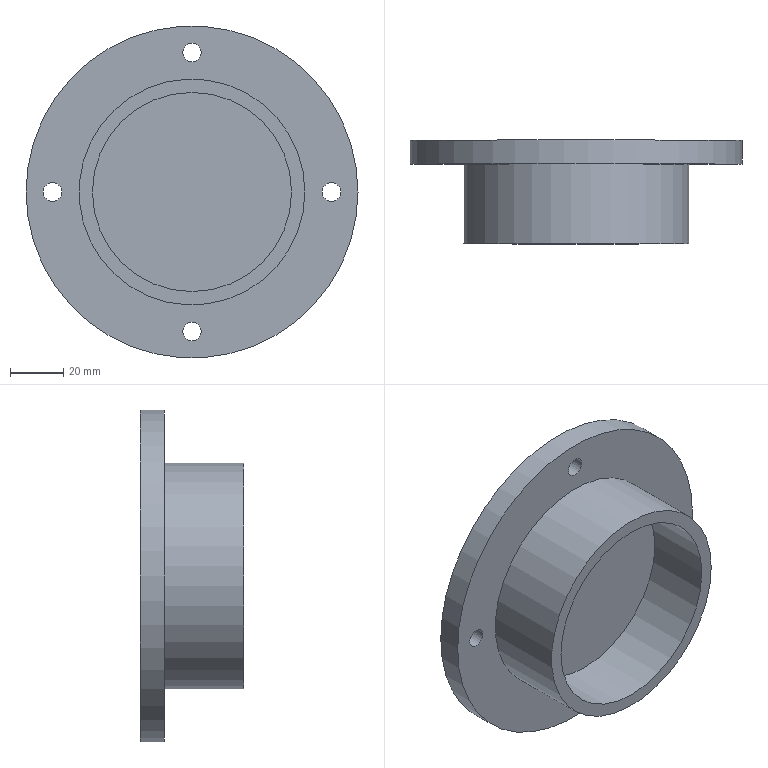Part | NX | features DATUM_CSYS 7, HOLE PACKAGE 6, SIMPLE HOLE 6, SKETCH 6, EXTRACT_DATUM_AXIS 4, Instance Feature 3, EXTRUDE 2, Pattern Feature 1 | 1 solid | 13 faces | box 125 x 39 x 125 mm | volume 158544 mm3 | cylinder 8 | plane 5 | commonest cylinder face diameters 7 x4 75 x1 81 x1 85 x1 125 x1
STEP:
#1=CARTESIAN_POINT('',(62.5,-9.,0.));
#2=VERTEX_POINT('',#1);
#3=CARTESIAN_POINT('',(0.,-9.,0.));
#4=DIRECTION('',(0.,-1.,0.));
#5=DIRECTION('',(1.,0.,0.));
#6=AXIS2_PLACEMENT_3D('',#3,#4,#5);
#7=CIRCLE('',#6,62.5);
#8=EDGE_CURVE('',#2,#2,#7,.T.);
#9=ORIENTED_EDGE('',*,*,#8,.F.);
#10=EDGE_LOOP('',(#9));
#11=FACE_BOUND('',#10,.T.);
#12=CARTESIAN_POINT('',(62.5,0.,0.));
#13=VERTEX_POINT('',#12);
#14=CARTESIAN_POINT('',(0.,0.,0.));
#15=DIRECTION('',(0.,-1.,0.));
#16=DIRECTION('',(1.,0.,0.));
#17=AXIS2_PLACEMENT_3D('',#14,#15,#16);
#18=CIRCLE('',#17,62.5);
#19=EDGE_CURVE('',#13,#13,#18,.T.);
#20=ORIENTED_EDGE('',*,*,#19,.T.);
#21=EDGE_LOOP('',(#20));
#22=FACE_BOUND('',#21,.T.);
#23=CARTESIAN_POINT('',(0.,-9.,0.));
#24=DIRECTION('',(0.,1.,0.));
#25=DIRECTION('',(0.,0.,1.));
#26=AXIS2_PLACEMENT_3D('',#23,#24,#25);
#27=CYLINDRICAL_SURFACE('',#26,62.5);
#28=ADVANCED_FACE('',(#11,#22),#27,.T.);
#29=CARTESIAN_POINT('',(0.,-9.,-56.));
#30=VERTEX_POINT('',#29);
#31=CARTESIAN_POINT('',(0.,-9.,-52.5));
#32=DIRECTION('',(0.,-1.,0.));
#33=DIRECTION('',(0.,0.,-1.));
#34=AXIS2_PLACEMENT_3D('',#31,#32,#33);
#35=CIRCLE('',#34,3.5);
#36=EDGE_CURVE('',#30,#30,#35,.T.);
#37=ORIENTED_EDGE('',*,*,#36,.F.);
#38=EDGE_LOOP('',(#37));
#39=FACE_BOUND('',#38,.T.);
#40=CARTESIAN_POINT('',(52.5,-9.,-3.5));
#41=VERTEX_POINT('',#40);
#42=CARTESIAN_POINT('',(52.5,-9.,0.));
#43=DIRECTION('',(0.,-1.,0.));
#44=DIRECTION('',(0.,0.,-1.));
#45=AXIS2_PLACEMENT_3D('',#42,#43,#44);
#46=CIRCLE('',#45,3.5);
#47=EDGE_CURVE('',#41,#41,#46,.T.);
#48=ORIENTED_EDGE('',*,*,#47,.F.);
#49=EDGE_LOOP('',(#48));
#50=FACE_BOUND('',#49,.T.);
#51=CARTESIAN_POINT('',(0.,-9.,49.));
#52=VERTEX_POINT('',#51);
#53=CARTESIAN_POINT('',(0.,-9.,52.5));
#54=DIRECTION('',(0.,-1.,0.));
#55=DIRECTION('',(0.,0.,-1.));
#56=AXIS2_PLACEMENT_3D('',#53,#54,#55);
#57=CIRCLE('',#56,3.5);
#58=EDGE_CURVE('',#52,#52,#57,.T.);
#59=ORIENTED_EDGE('',*,*,#58,.F.);
#60=EDGE_LOOP('',(#59));
#61=FACE_BOUND('',#60,.T.);
#62=CARTESIAN_POINT('',(-52.5,-9.,-3.5));
#63=VERTEX_POINT('',#62);
#64=CARTESIAN_POINT('',(-52.5,-9.,0.));
#65=DIRECTION('',(0.,-1.,0.));
#66=DIRECTION('',(0.,0.,-1.));
#67=AXIS2_PLACEMENT_3D('',#64,#65,#66);
#68=CIRCLE('',#67,3.5);
#69=EDGE_CURVE('',#63,#63,#68,.T.);
#70=ORIENTED_EDGE('',*,*,#69,.F.);
#71=EDGE_LOOP('',(#70));
#72=FACE_BOUND('',#71,.T.);
#73=CARTESIAN_POINT('',(42.5,-9.,0.));
#74=VERTEX_POINT('',#73);
#75=CARTESIAN_POINT('',(0.,-9.,0.));
#76=DIRECTION('',(0.,-1.,0.));
#77=DIRECTION('',(1.,0.,0.));
#78=AXIS2_PLACEMENT_3D('',#75,#76,#77);
#79=CIRCLE('',#78,42.5);
#80=EDGE_CURVE('',#74,#74,#79,.T.);
#81=ORIENTED_EDGE('',*,*,#80,.F.);
#82=EDGE_LOOP('',(#81));
#83=FACE_BOUND('',#82,.T.);
#84=ORIENTED_EDGE('',*,*,#8,.T.);
#85=EDGE_LOOP('',(#84));
#86=FACE_BOUND('',#85,.T.);
#87=CARTESIAN_POINT('',(0.,-9.,0.));
#88=DIRECTION('',(0.,-1.,0.));
#89=DIRECTION('',(0.,0.,-1.));
#90=AXIS2_PLACEMENT_3D('',#87,#88,#89);
#91=PLANE('',#90);
#92=ADVANCED_FACE('',(#39,#50,#61,#72,#83,#86),#91,.T.);
#93=CARTESIAN_POINT('',(0.,0.,-40.5));
#94=VERTEX_POINT('',#93);
#95=CARTESIAN_POINT('',(0.,0.,0.));
#96=DIRECTION('',(0.,-1.,0.));
#97=DIRECTION('',(0.,0.,-1.));
#98=AXIS2_PLACEMENT_3D('',#95,#96,#97);
#99=CIRCLE('',#98,40.5);
#100=EDGE_CURVE('',#94,#94,#99,.T.);
#101=ORIENTED_EDGE('',*,*,#100,.T.);
#102=EDGE_LOOP('',(#101));
#103=FACE_BOUND('',#102,.T.);
#104=CARTESIAN_POINT('',(0.,0.,-56.));
#105=VERTEX_POINT('',#104);
#106=CARTESIAN_POINT('',(0.,0.,-52.5));
#107=DIRECTION('',(0.,-1.,0.));
#108=DIRECTION('',(0.,0.,-1.));
#109=AXIS2_PLACEMENT_3D('',#106,#107,#108);
#110=CIRCLE('',#109,3.5);
#111=EDGE_CURVE('',#105,#105,#110,.T.);
#112=ORIENTED_EDGE('',*,*,#111,.T.);
#113=EDGE_LOOP('',(#112));
#114=FACE_BOUND('',#113,.T.);
#115=CARTESIAN_POINT('',(52.5,0.,-3.5));
#116=VERTEX_POINT('',#115);
#117=CARTESIAN_POINT('',(52.5,0.,0.));
#118=DIRECTION('',(0.,-1.,0.));
#119=DIRECTION('',(0.,0.,-1.));
#120=AXIS2_PLACEMENT_3D('',#117,#118,#119);
#121=CIRCLE('',#120,3.5);
#122=EDGE_CURVE('',#116,#116,#121,.T.);
#123=ORIENTED_EDGE('',*,*,#122,.T.);
#124=EDGE_LOOP('',(#123));
#125=FACE_BOUND('',#124,.T.);
#126=CARTESIAN_POINT('',(0.,0.,49.));
#127=VERTEX_POINT('',#126);
#128=CARTESIAN_POINT('',(0.,0.,52.5));
#129=DIRECTION('',(0.,-1.,0.));
#130=DIRECTION('',(0.,0.,-1.));
#131=AXIS2_PLACEMENT_3D('',#128,#129,#130);
#132=CIRCLE('',#131,3.5);
#133=EDGE_CURVE('',#127,#127,#132,.T.);
#134=ORIENTED_EDGE('',*,*,#133,.T.);
#135=EDGE_LOOP('',(#134));
#136=FACE_BOUND('',#135,.T.);
#137=CARTESIAN_POINT('',(-52.5,0.,-3.5));
#138=VERTEX_POINT('',#137);
#139=CARTESIAN_POINT('',(-52.5,0.,0.));
#140=DIRECTION('',(0.,-1.,0.));
#141=DIRECTION('',(0.,0.,-1.));
#142=AXIS2_PLACEMENT_3D('',#139,#140,#141);
#143=CIRCLE('',#142,3.5);
#144=EDGE_CURVE('',#138,#138,#143,.T.);
#145=ORIENTED_EDGE('',*,*,#144,.T.);
#146=EDGE_LOOP('',(#145));
#147=FACE_BOUND('',#146,.T.);
#148=ORIENTED_EDGE('',*,*,#19,.F.);
#149=EDGE_LOOP('',(#148));
#150=FACE_BOUND('',#149,.T.);
#151=CARTESIAN_POINT('',(0.,0.,0.));
#152=DIRECTION('',(0.,-1.,0.));
#153=DIRECTION('',(0.,0.,-1.));
#154=AXIS2_PLACEMENT_3D('',#151,#152,#153);
#155=PLANE('',#154);
#156=ADVANCED_FACE('',(#103,#114,#125,#136,#147,#150),#155,.F.);
#157=CARTESIAN_POINT('',(42.5,-39.,0.));
#158=VERTEX_POINT('',#157);
#159=CARTESIAN_POINT('',(0.,-39.,0.));
#160=DIRECTION('',(0.,-1.,0.));
#161=DIRECTION('',(1.,0.,0.));
#162=AXIS2_PLACEMENT_3D('',#159,#160,#161);
#163=CIRCLE('',#162,42.5);
#164=EDGE_CURVE('',#158,#158,#163,.T.);
#165=ORIENTED_EDGE('',*,*,#164,.F.);
#166=EDGE_LOOP('',(#165));
#167=FACE_BOUND('',#166,.T.);
#168=ORIENTED_EDGE('',*,*,#80,.T.);
#169=EDGE_LOOP('',(#168));
#170=FACE_BOUND('',#169,.T.);
#171=CARTESIAN_POINT('',(0.,-39.,0.));
#172=DIRECTION('',(0.,1.,0.));
#173=DIRECTION('',(0.,0.,1.));
#174=AXIS2_PLACEMENT_3D('',#171,#172,#173);
#175=CYLINDRICAL_SURFACE('',#174,42.5);
#176=ADVANCED_FACE('',(#167,#170),#175,.T.);
#177=CARTESIAN_POINT('',(0.,-39.,37.5));
#178=VERTEX_POINT('',#177);
#179=CARTESIAN_POINT('',(0.,-39.,0.));
#180=DIRECTION('',(0.,1.,0.));
#181=DIRECTION('',(0.,0.,1.));
#182=AXIS2_PLACEMENT_3D('',#179,#180,#181);
#183=CIRCLE('',#182,37.5);
#184=EDGE_CURVE('',#178,#178,#183,.T.);
#185=ORIENTED_EDGE('',*,*,#184,.T.);
#186=EDGE_LOOP('',(#185));
#187=FACE_BOUND('',#186,.T.);
#188=ORIENTED_EDGE('',*,*,#164,.T.);
#189=EDGE_LOOP('',(#188));
#190=FACE_BOUND('',#189,.T.);
#191=CARTESIAN_POINT('',(0.,-39.,0.));
#192=DIRECTION('',(0.,-1.,0.));
#193=DIRECTION('',(0.,0.,-1.));
#194=AXIS2_PLACEMENT_3D('',#191,#192,#193);
#195=PLANE('',#194);
#196=ADVANCED_FACE('',(#187,#190),#195,.T.);
#197=CARTESIAN_POINT('',(0.,-14.,37.5));
#198=VERTEX_POINT('',#197);
#199=CARTESIAN_POINT('',(0.,-14.,0.));
#200=DIRECTION('',(0.,1.,0.));
#201=DIRECTION('',(0.,0.,1.));
#202=AXIS2_PLACEMENT_3D('',#199,#200,#201);
#203=CIRCLE('',#202,37.5);
#204=EDGE_CURVE('',#198,#198,#203,.F.);
#205=ORIENTED_EDGE('',*,*,#204,.T.);
#206=EDGE_LOOP('',(#205));
#207=FACE_BOUND('',#206,.T.);
#208=CARTESIAN_POINT('',(0.,-14.,0.));
#209=DIRECTION('',(0.,1.,0.));
#210=DIRECTION('',(0.,0.,1.));
#211=AXIS2_PLACEMENT_3D('',#208,#209,#210);
#212=PLANE('',#211);
#213=ADVANCED_FACE('',(#207),#212,.F.);
#214=ORIENTED_EDGE('',*,*,#204,.F.);
#215=EDGE_LOOP('',(#214));
#216=FACE_BOUND('',#215,.T.);
#217=ORIENTED_EDGE('',*,*,#184,.F.);
#218=EDGE_LOOP('',(#217));
#219=FACE_BOUND('',#218,.T.);
#220=CARTESIAN_POINT('',(0.,-39.,0.));
#221=DIRECTION('',(0.,1.,0.));
#222=DIRECTION('',(0.,0.,1.));
#223=AXIS2_PLACEMENT_3D('',#220,#221,#222);
#224=CYLINDRICAL_SURFACE('',#223,37.5);
#225=ADVANCED_FACE('',(#216,#219),#224,.F.);
#226=ORIENTED_EDGE('',*,*,#69,.T.);
#227=EDGE_LOOP('',(#226));
#228=FACE_BOUND('',#227,.T.);
#229=ORIENTED_EDGE('',*,*,#144,.F.);
#230=EDGE_LOOP('',(#229));
#231=FACE_BOUND('',#230,.T.);
#232=CARTESIAN_POINT('',(-52.5,0.,0.));
#233=DIRECTION('',(0.,-1.,0.));
#234=DIRECTION('',(0.,0.,-1.));
#235=AXIS2_PLACEMENT_3D('',#232,#233,#234);
#236=CYLINDRICAL_SURFACE('',#235,3.5);
#237=ADVANCED_FACE('',(#228,#231),#236,.F.);
#238=ORIENTED_EDGE('',*,*,#58,.T.);
#239=EDGE_LOOP('',(#238));
#240=FACE_BOUND('',#239,.T.);
#241=ORIENTED_EDGE('',*,*,#133,.F.);
#242=EDGE_LOOP('',(#241));
#243=FACE_BOUND('',#242,.T.);
#244=CARTESIAN_POINT('',(0.,0.,52.5));
#245=DIRECTION('',(0.,-1.,0.));
#246=DIRECTION('',(0.,0.,-1.));
#247=AXIS2_PLACEMENT_3D('',#244,#245,#246);
#248=CYLINDRICAL_SURFACE('',#247,3.5);
#249=ADVANCED_FACE('',(#240,#243),#248,.F.);
#250=ORIENTED_EDGE('',*,*,#47,.T.);
#251=EDGE_LOOP('',(#250));
#252=FACE_BOUND('',#251,.T.);
#253=ORIENTED_EDGE('',*,*,#122,.F.);
#254=EDGE_LOOP('',(#253));
#255=FACE_BOUND('',#254,.T.);
#256=CARTESIAN_POINT('',(52.5,0.,0.));
#257=DIRECTION('',(0.,-1.,0.));
#258=DIRECTION('',(0.,0.,-1.));
#259=AXIS2_PLACEMENT_3D('',#256,#257,#258);
#260=CYLINDRICAL_SURFACE('',#259,3.5);
#261=ADVANCED_FACE('',(#252,#255),#260,.F.);
#262=ORIENTED_EDGE('',*,*,#36,.T.);
#263=EDGE_LOOP('',(#262));
#264=FACE_BOUND('',#263,.T.);
#265=ORIENTED_EDGE('',*,*,#111,.F.);
#266=EDGE_LOOP('',(#265));
#267=FACE_BOUND('',#266,.T.);
#268=CARTESIAN_POINT('',(0.,0.,-52.5));
#269=DIRECTION('',(0.,-1.,0.));
#270=DIRECTION('',(0.,0.,-1.));
#271=AXIS2_PLACEMENT_3D('',#268,#269,#270);
#272=CYLINDRICAL_SURFACE('',#271,3.5);
#273=ADVANCED_FACE('',(#264,#267),#272,.F.);
#274=CARTESIAN_POINT('',(0.,-2.,-40.5));
#275=VERTEX_POINT('',#274);
#276=CARTESIAN_POINT('',(0.,-2.,0.));
#277=DIRECTION('',(0.,-1.,0.));
#278=DIRECTION('',(0.,0.,-1.));
#279=AXIS2_PLACEMENT_3D('',#276,#277,#278);
#280=CIRCLE('',#279,40.5);
#281=EDGE_CURVE('',#275,#275,#280,.F.);
#282=ORIENTED_EDGE('',*,*,#281,.T.);
#283=EDGE_LOOP('',(#282));
#284=FACE_BOUND('',#283,.T.);
#285=CARTESIAN_POINT('',(0.,-2.,0.));
#286=DIRECTION('',(0.,-1.,0.));
#287=DIRECTION('',(0.,0.,-1.));
#288=AXIS2_PLACEMENT_3D('',#285,#286,#287);
#289=PLANE('',#288);
#290=ADVANCED_FACE('',(#284),#289,.F.);
#291=ORIENTED_EDGE('',*,*,#281,.F.);
#292=EDGE_LOOP('',(#291));
#293=FACE_BOUND('',#292,.T.);
#294=ORIENTED_EDGE('',*,*,#100,.F.);
#295=EDGE_LOOP('',(#294));
#296=FACE_BOUND('',#295,.T.);
#297=CARTESIAN_POINT('',(0.,0.,0.));
#298=DIRECTION('',(0.,-1.,0.));
#299=DIRECTION('',(0.,0.,-1.));
#300=AXIS2_PLACEMENT_3D('',#297,#298,#299);
#301=CYLINDRICAL_SURFACE('',#300,40.5);
#302=ADVANCED_FACE('',(#293,#296),#301,.F.);
#303=CLOSED_SHELL('',(#28,#92,#156,#176,#196,#213,#225,#237,#249,#261,#273,#290,#302));
#304=MANIFOLD_SOLID_BREP('',#303);
#305=(LENGTH_UNIT()NAMED_UNIT(*)SI_UNIT(.MILLI.,.METRE.));
#306=UNCERTAINTY_MEASURE_WITH_UNIT(LENGTH_MEASURE(0.00001),#305,'','');
#307=(NAMED_UNIT(*)PLANE_ANGLE_UNIT()SI_UNIT($,.RADIAN.));
#308=(NAMED_UNIT(*)SI_UNIT($,.STERADIAN.)SOLID_ANGLE_UNIT());
#309=(GEOMETRIC_REPRESENTATION_CONTEXT(3)GLOBAL_UNCERTAINTY_ASSIGNED_CONTEXT((#306))GLOBAL_UNIT_ASSIGNED_CONTEXT((#305,#307,#308))REPRESENTATION_CONTEXT('',''));
#310=ADVANCED_BREP_SHAPE_REPRESENTATION('',(#304),#309);